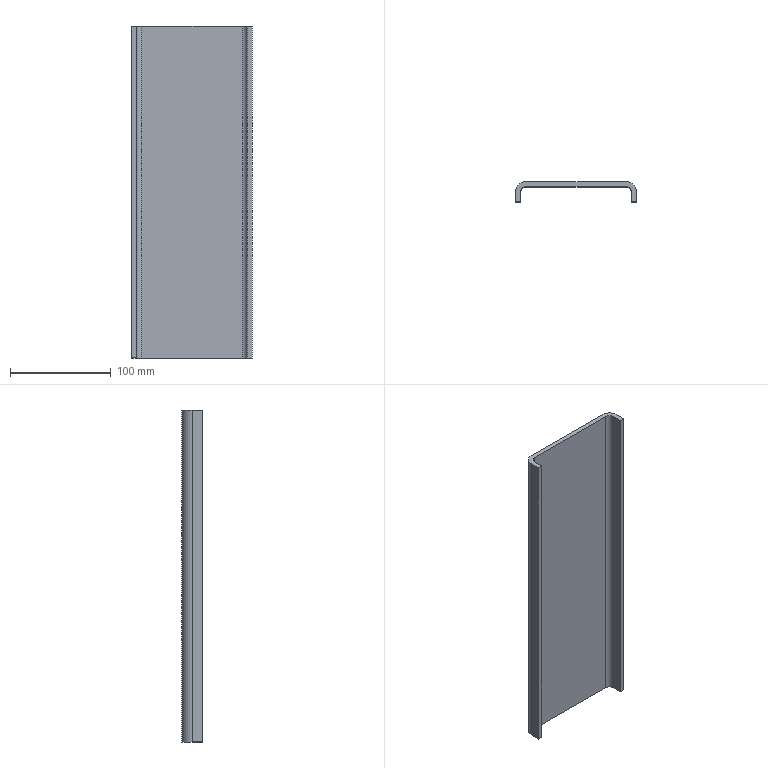Part | SolidWorks | features Extrusion 1, ICE 1 | 1 solid | 14 faces | box 120 x 20 x 330 mm | volume 236877 mm3 | plane 10 | cylinder 4 | commonest cylinder face diameters 10 x2 20 x2
STEP:
#1=CARTESIAN_POINT('',(115.,-20.,320.));
#2=VERTEX_POINT('',#1);
#3=CARTESIAN_POINT('',(115.,-20.,-10.));
#4=VERTEX_POINT('',#3);
#5=CARTESIAN_POINT('',(115.,-20.,320.));
#6=DIRECTION('',(0.,0.,-1.));
#7=VECTOR('',#6,1000.);
#8=LINE('',#5,#7);
#9=EDGE_CURVE('',#2,#4,#8,.T.);
#10=ORIENTED_EDGE('',*,*,#9,.T.);
#11=CARTESIAN_POINT('',(120.,-20.,-10.));
#12=VERTEX_POINT('',#11);
#13=CARTESIAN_POINT('',(120.,-20.,-10.));
#14=DIRECTION('',(-1.,0.,0.));
#15=VECTOR('',#14,1000.);
#16=LINE('',#13,#15);
#17=EDGE_CURVE('',#12,#4,#16,.T.);
#18=ORIENTED_EDGE('',*,*,#17,.F.);
#19=CARTESIAN_POINT('',(120.,-20.,320.));
#20=VERTEX_POINT('',#19);
#21=CARTESIAN_POINT('',(120.,-20.,320.));
#22=DIRECTION('',(0.,0.,-1.));
#23=VECTOR('',#22,1000.);
#24=LINE('',#21,#23);
#25=EDGE_CURVE('',#20,#12,#24,.T.);
#26=ORIENTED_EDGE('',*,*,#25,.F.);
#27=CARTESIAN_POINT('',(115.,-20.,320.));
#28=DIRECTION('',(1.,0.,0.));
#29=VECTOR('',#28,1000.);
#30=LINE('',#27,#29);
#31=EDGE_CURVE('',#2,#20,#30,.T.);
#32=ORIENTED_EDGE('',*,*,#31,.F.);
#33=EDGE_LOOP('',(#10,#18,#26,#32));
#34=FACE_OUTER_BOUND('',#33,.T.);
#35=CARTESIAN_POINT('',(115.,-20.,320.));
#36=DIRECTION('',(0.,1.,0.));
#37=DIRECTION('',(0.,0.,1.));
#38=AXIS2_PLACEMENT_3D('',#35,#36,#37);
#39=PLANE('',#38);
#40=ADVANCED_FACE('',(#34),#39,.F.);
#41=ORIENTED_EDGE('',*,*,#25,.T.);
#42=CARTESIAN_POINT('',(120.,-10.,-10.));
#43=VERTEX_POINT('',#42);
#44=CARTESIAN_POINT('',(120.,-10.,-10.));
#45=DIRECTION('',(0.,-1.,0.));
#46=VECTOR('',#45,1000.);
#47=LINE('',#44,#46);
#48=EDGE_CURVE('',#43,#12,#47,.T.);
#49=ORIENTED_EDGE('',*,*,#48,.F.);
#50=CARTESIAN_POINT('',(120.,-10.,320.));
#51=VERTEX_POINT('',#50);
#52=CARTESIAN_POINT('',(120.,-10.,320.));
#53=DIRECTION('',(0.,0.,-1.));
#54=VECTOR('',#53,1000.);
#55=LINE('',#52,#54);
#56=EDGE_CURVE('',#51,#43,#55,.T.);
#57=ORIENTED_EDGE('',*,*,#56,.F.);
#58=CARTESIAN_POINT('',(120.,-10.,320.));
#59=DIRECTION('',(0.,1.,0.));
#60=VECTOR('',#59,1000.);
#61=LINE('',#58,#60);
#62=EDGE_CURVE('',#20,#51,#61,.T.);
#63=ORIENTED_EDGE('',*,*,#62,.F.);
#64=EDGE_LOOP('',(#41,#49,#57,#63));
#65=FACE_OUTER_BOUND('',#64,.T.);
#66=CARTESIAN_POINT('',(120.,-10.,320.));
#67=DIRECTION('',(-1.,0.,0.));
#68=DIRECTION('',(0.,0.,1.));
#69=AXIS2_PLACEMENT_3D('',#66,#67,#68);
#70=PLANE('',#69);
#71=ADVANCED_FACE('',(#65),#70,.F.);
#72=ORIENTED_EDGE('',*,*,#56,.T.);
#73=CARTESIAN_POINT('',(110.,0.,-10.));
#74=VERTEX_POINT('',#73);
#75=CARTESIAN_POINT('',(110.,-10.,-10.));
#76=DIRECTION('',(0.,0.,-1.));
#77=DIRECTION('',(-1.,0.,0.));
#78=AXIS2_PLACEMENT_3D('',#75,#76,#77);
#79=CIRCLE('',#78,10.);
#80=EDGE_CURVE('',#74,#43,#79,.T.);
#81=ORIENTED_EDGE('',*,*,#80,.F.);
#82=CARTESIAN_POINT('',(110.,0.,320.));
#83=VERTEX_POINT('',#82);
#84=CARTESIAN_POINT('',(110.,0.,320.));
#85=DIRECTION('',(0.,0.,-1.));
#86=VECTOR('',#85,1000.);
#87=LINE('',#84,#86);
#88=EDGE_CURVE('',#83,#74,#87,.T.);
#89=ORIENTED_EDGE('',*,*,#88,.F.);
#90=CARTESIAN_POINT('',(110.,-10.,320.));
#91=DIRECTION('',(0.,0.,1.));
#92=DIRECTION('',(1.,0.,0.));
#93=AXIS2_PLACEMENT_3D('',#90,#91,#92);
#94=CIRCLE('',#93,10.);
#95=EDGE_CURVE('',#51,#83,#94,.T.);
#96=ORIENTED_EDGE('',*,*,#95,.F.);
#97=EDGE_LOOP('',(#72,#81,#89,#96));
#98=FACE_OUTER_BOUND('',#97,.T.);
#99=CARTESIAN_POINT('',(110.,-10.,320.));
#100=DIRECTION('',(0.,0.,-1.));
#101=DIRECTION('',(-1.,0.,0.));
#102=AXIS2_PLACEMENT_3D('',#99,#100,#101);
#103=CYLINDRICAL_SURFACE('',#102,10.);
#104=ADVANCED_FACE('',(#98),#103,.T.);
#105=ORIENTED_EDGE('',*,*,#88,.T.);
#106=CARTESIAN_POINT('',(10.,0.,-10.));
#107=VERTEX_POINT('',#106);
#108=CARTESIAN_POINT('',(10.,0.,-10.));
#109=DIRECTION('',(1.,0.,0.));
#110=VECTOR('',#109,1000.);
#111=LINE('',#108,#110);
#112=EDGE_CURVE('',#107,#74,#111,.T.);
#113=ORIENTED_EDGE('',*,*,#112,.F.);
#114=CARTESIAN_POINT('',(10.,0.,320.));
#115=VERTEX_POINT('',#114);
#116=CARTESIAN_POINT('',(10.,0.,320.));
#117=DIRECTION('',(0.,0.,-1.));
#118=VECTOR('',#117,1000.);
#119=LINE('',#116,#118);
#120=EDGE_CURVE('',#115,#107,#119,.T.);
#121=ORIENTED_EDGE('',*,*,#120,.F.);
#122=CARTESIAN_POINT('',(10.,0.,320.));
#123=DIRECTION('',(-1.,0.,0.));
#124=VECTOR('',#123,1000.);
#125=LINE('',#122,#124);
#126=EDGE_CURVE('',#83,#115,#125,.T.);
#127=ORIENTED_EDGE('',*,*,#126,.F.);
#128=EDGE_LOOP('',(#105,#113,#121,#127));
#129=FACE_OUTER_BOUND('',#128,.T.);
#130=CARTESIAN_POINT('',(10.,0.,320.));
#131=DIRECTION('',(0.,-1.,0.));
#132=DIRECTION('',(0.,0.,-1.));
#133=AXIS2_PLACEMENT_3D('',#130,#131,#132);
#134=PLANE('',#133);
#135=ADVANCED_FACE('',(#129),#134,.F.);
#136=ORIENTED_EDGE('',*,*,#120,.T.);
#137=CARTESIAN_POINT('',(0.,-10.,-10.));
#138=VERTEX_POINT('',#137);
#139=CARTESIAN_POINT('',(10.,-10.,-10.));
#140=DIRECTION('',(0.,0.,-1.));
#141=DIRECTION('',(-1.,0.,0.));
#142=AXIS2_PLACEMENT_3D('',#139,#140,#141);
#143=CIRCLE('',#142,10.);
#144=EDGE_CURVE('',#138,#107,#143,.T.);
#145=ORIENTED_EDGE('',*,*,#144,.F.);
#146=CARTESIAN_POINT('',(0.,-10.,320.));
#147=VERTEX_POINT('',#146);
#148=CARTESIAN_POINT('',(0.,-10.,320.));
#149=DIRECTION('',(0.,0.,-1.));
#150=VECTOR('',#149,1000.);
#151=LINE('',#148,#150);
#152=EDGE_CURVE('',#147,#138,#151,.T.);
#153=ORIENTED_EDGE('',*,*,#152,.F.);
#154=CARTESIAN_POINT('',(10.,-10.,320.));
#155=DIRECTION('',(0.,0.,1.));
#156=DIRECTION('',(1.,0.,0.));
#157=AXIS2_PLACEMENT_3D('',#154,#155,#156);
#158=CIRCLE('',#157,10.);
#159=EDGE_CURVE('',#115,#147,#158,.T.);
#160=ORIENTED_EDGE('',*,*,#159,.F.);
#161=EDGE_LOOP('',(#136,#145,#153,#160));
#162=FACE_OUTER_BOUND('',#161,.T.);
#163=CARTESIAN_POINT('',(10.,-10.,320.));
#164=DIRECTION('',(0.,0.,-1.));
#165=DIRECTION('',(-1.,0.,0.));
#166=AXIS2_PLACEMENT_3D('',#163,#164,#165);
#167=CYLINDRICAL_SURFACE('',#166,10.);
#168=ADVANCED_FACE('',(#162),#167,.T.);
#169=ORIENTED_EDGE('',*,*,#152,.T.);
#170=CARTESIAN_POINT('',(0.,-20.,-10.));
#171=VERTEX_POINT('',#170);
#172=CARTESIAN_POINT('',(0.,-20.,-10.));
#173=DIRECTION('',(0.,1.,0.));
#174=VECTOR('',#173,1000.);
#175=LINE('',#172,#174);
#176=EDGE_CURVE('',#171,#138,#175,.T.);
#177=ORIENTED_EDGE('',*,*,#176,.F.);
#178=CARTESIAN_POINT('',(0.,-20.,320.));
#179=VERTEX_POINT('',#178);
#180=CARTESIAN_POINT('',(0.,-20.,320.));
#181=DIRECTION('',(0.,0.,-1.));
#182=VECTOR('',#181,1000.);
#183=LINE('',#180,#182);
#184=EDGE_CURVE('',#179,#171,#183,.T.);
#185=ORIENTED_EDGE('',*,*,#184,.F.);
#186=CARTESIAN_POINT('',(0.,-10.,320.));
#187=DIRECTION('',(0.,-1.,0.));
#188=VECTOR('',#187,1000.);
#189=LINE('',#186,#188);
#190=EDGE_CURVE('',#147,#179,#189,.T.);
#191=ORIENTED_EDGE('',*,*,#190,.F.);
#192=EDGE_LOOP('',(#169,#177,#185,#191));
#193=FACE_OUTER_BOUND('',#192,.T.);
#194=CARTESIAN_POINT('',(0.,-10.,320.));
#195=DIRECTION('',(1.,0.,0.));
#196=DIRECTION('',(0.,1.,0.));
#197=AXIS2_PLACEMENT_3D('',#194,#195,#196);
#198=PLANE('',#197);
#199=ADVANCED_FACE('',(#193),#198,.F.);
#200=ORIENTED_EDGE('',*,*,#184,.T.);
#201=CARTESIAN_POINT('',(5.,-20.,-10.));
#202=VERTEX_POINT('',#201);
#203=CARTESIAN_POINT('',(5.,-20.,-10.));
#204=DIRECTION('',(-1.,0.,0.));
#205=VECTOR('',#204,1000.);
#206=LINE('',#203,#205);
#207=EDGE_CURVE('',#202,#171,#206,.T.);
#208=ORIENTED_EDGE('',*,*,#207,.F.);
#209=CARTESIAN_POINT('',(5.,-20.,320.));
#210=VERTEX_POINT('',#209);
#211=CARTESIAN_POINT('',(5.,-20.,320.));
#212=DIRECTION('',(0.,0.,-1.));
#213=VECTOR('',#212,1000.);
#214=LINE('',#211,#213);
#215=EDGE_CURVE('',#210,#202,#214,.T.);
#216=ORIENTED_EDGE('',*,*,#215,.F.);
#217=CARTESIAN_POINT('',(0.,-20.,320.));
#218=DIRECTION('',(1.,0.,0.));
#219=VECTOR('',#218,1000.);
#220=LINE('',#217,#219);
#221=EDGE_CURVE('',#179,#210,#220,.T.);
#222=ORIENTED_EDGE('',*,*,#221,.F.);
#223=EDGE_LOOP('',(#200,#208,#216,#222));
#224=FACE_OUTER_BOUND('',#223,.T.);
#225=CARTESIAN_POINT('',(0.,-20.,320.));
#226=DIRECTION('',(0.,1.,0.));
#227=DIRECTION('',(0.,0.,1.));
#228=AXIS2_PLACEMENT_3D('',#225,#226,#227);
#229=PLANE('',#228);
#230=ADVANCED_FACE('',(#224),#229,.F.);
#231=ORIENTED_EDGE('',*,*,#215,.T.);
#232=CARTESIAN_POINT('',(5.,-10.,-10.));
#233=VERTEX_POINT('',#232);
#234=CARTESIAN_POINT('',(5.,-10.,-10.));
#235=DIRECTION('',(0.,-1.,0.));
#236=VECTOR('',#235,1000.);
#237=LINE('',#234,#236);
#238=EDGE_CURVE('',#233,#202,#237,.T.);
#239=ORIENTED_EDGE('',*,*,#238,.F.);
#240=CARTESIAN_POINT('',(5.,-10.,320.));
#241=VERTEX_POINT('',#240);
#242=CARTESIAN_POINT('',(5.,-10.,320.));
#243=DIRECTION('',(0.,0.,-1.));
#244=VECTOR('',#243,1000.);
#245=LINE('',#242,#244);
#246=EDGE_CURVE('',#241,#233,#245,.T.);
#247=ORIENTED_EDGE('',*,*,#246,.F.);
#248=CARTESIAN_POINT('',(5.,-10.,320.));
#249=DIRECTION('',(0.,1.,0.));
#250=VECTOR('',#249,1000.);
#251=LINE('',#248,#250);
#252=EDGE_CURVE('',#210,#241,#251,.T.);
#253=ORIENTED_EDGE('',*,*,#252,.F.);
#254=EDGE_LOOP('',(#231,#239,#247,#253));
#255=FACE_OUTER_BOUND('',#254,.T.);
#256=CARTESIAN_POINT('',(5.,-10.,320.));
#257=DIRECTION('',(-1.,0.,0.));
#258=DIRECTION('',(0.,0.,1.));
#259=AXIS2_PLACEMENT_3D('',#256,#257,#258);
#260=PLANE('',#259);
#261=ADVANCED_FACE('',(#255),#260,.F.);
#262=ORIENTED_EDGE('',*,*,#246,.T.);
#263=CARTESIAN_POINT('',(10.,-5.,-10.));
#264=VERTEX_POINT('',#263);
#265=CARTESIAN_POINT('',(10.,-10.,-10.));
#266=DIRECTION('',(0.,0.,1.));
#267=DIRECTION('',(-1.,0.,0.));
#268=AXIS2_PLACEMENT_3D('',#265,#266,#267);
#269=CIRCLE('',#268,5.);
#270=EDGE_CURVE('',#264,#233,#269,.T.);
#271=ORIENTED_EDGE('',*,*,#270,.F.);
#272=CARTESIAN_POINT('',(10.,-5.,320.));
#273=VERTEX_POINT('',#272);
#274=CARTESIAN_POINT('',(10.,-5.,320.));
#275=DIRECTION('',(0.,0.,-1.));
#276=VECTOR('',#275,1000.);
#277=LINE('',#274,#276);
#278=EDGE_CURVE('',#273,#264,#277,.T.);
#279=ORIENTED_EDGE('',*,*,#278,.F.);
#280=CARTESIAN_POINT('',(10.,-10.,320.));
#281=DIRECTION('',(0.,0.,-1.));
#282=DIRECTION('',(1.,0.,0.));
#283=AXIS2_PLACEMENT_3D('',#280,#281,#282);
#284=CIRCLE('',#283,5.);
#285=EDGE_CURVE('',#241,#273,#284,.T.);
#286=ORIENTED_EDGE('',*,*,#285,.F.);
#287=EDGE_LOOP('',(#262,#271,#279,#286));
#288=FACE_OUTER_BOUND('',#287,.T.);
#289=CARTESIAN_POINT('',(10.,-10.,320.));
#290=DIRECTION('',(0.,0.,-1.));
#291=DIRECTION('',(-1.,0.,0.));
#292=AXIS2_PLACEMENT_3D('',#289,#290,#291);
#293=CYLINDRICAL_SURFACE('',#292,5.);
#294=ADVANCED_FACE('',(#288),#293,.F.);
#295=ORIENTED_EDGE('',*,*,#278,.T.);
#296=CARTESIAN_POINT('',(110.,-5.,-10.));
#297=VERTEX_POINT('',#296);
#298=CARTESIAN_POINT('',(110.,-5.,-10.));
#299=DIRECTION('',(-1.,0.,0.));
#300=VECTOR('',#299,1000.);
#301=LINE('',#298,#300);
#302=EDGE_CURVE('',#297,#264,#301,.T.);
#303=ORIENTED_EDGE('',*,*,#302,.F.);
#304=CARTESIAN_POINT('',(110.,-5.,320.));
#305=VERTEX_POINT('',#304);
#306=CARTESIAN_POINT('',(110.,-5.,320.));
#307=DIRECTION('',(0.,0.,-1.));
#308=VECTOR('',#307,1000.);
#309=LINE('',#306,#308);
#310=EDGE_CURVE('',#305,#297,#309,.T.);
#311=ORIENTED_EDGE('',*,*,#310,.F.);
#312=CARTESIAN_POINT('',(10.,-5.,320.));
#313=DIRECTION('',(1.,0.,0.));
#314=VECTOR('',#313,1000.);
#315=LINE('',#312,#314);
#316=EDGE_CURVE('',#273,#305,#315,.T.);
#317=ORIENTED_EDGE('',*,*,#316,.F.);
#318=EDGE_LOOP('',(#295,#303,#311,#317));
#319=FACE_OUTER_BOUND('',#318,.T.);
#320=CARTESIAN_POINT('',(10.,-5.,320.));
#321=DIRECTION('',(0.,1.,0.));
#322=DIRECTION('',(0.,0.,1.));
#323=AXIS2_PLACEMENT_3D('',#320,#321,#322);
#324=PLANE('',#323);
#325=ADVANCED_FACE('',(#319),#324,.F.);
#326=ORIENTED_EDGE('',*,*,#310,.T.);
#327=CARTESIAN_POINT('',(115.,-10.,-10.));
#328=VERTEX_POINT('',#327);
#329=CARTESIAN_POINT('',(110.,-10.,-10.));
#330=DIRECTION('',(0.,0.,1.));
#331=DIRECTION('',(-1.,0.,0.));
#332=AXIS2_PLACEMENT_3D('',#329,#330,#331);
#333=CIRCLE('',#332,5.);
#334=EDGE_CURVE('',#328,#297,#333,.T.);
#335=ORIENTED_EDGE('',*,*,#334,.F.);
#336=CARTESIAN_POINT('',(115.,-10.,320.));
#337=VERTEX_POINT('',#336);
#338=CARTESIAN_POINT('',(115.,-10.,320.));
#339=DIRECTION('',(0.,0.,-1.));
#340=VECTOR('',#339,1000.);
#341=LINE('',#338,#340);
#342=EDGE_CURVE('',#337,#328,#341,.T.);
#343=ORIENTED_EDGE('',*,*,#342,.F.);
#344=CARTESIAN_POINT('',(110.,-10.,320.));
#345=DIRECTION('',(0.,0.,-1.));
#346=DIRECTION('',(1.,0.,0.));
#347=AXIS2_PLACEMENT_3D('',#344,#345,#346);
#348=CIRCLE('',#347,5.);
#349=EDGE_CURVE('',#305,#337,#348,.T.);
#350=ORIENTED_EDGE('',*,*,#349,.F.);
#351=EDGE_LOOP('',(#326,#335,#343,#350));
#352=FACE_OUTER_BOUND('',#351,.T.);
#353=CARTESIAN_POINT('',(110.,-10.,320.));
#354=DIRECTION('',(0.,0.,-1.));
#355=DIRECTION('',(-1.,0.,0.));
#356=AXIS2_PLACEMENT_3D('',#353,#354,#355);
#357=CYLINDRICAL_SURFACE('',#356,5.);
#358=ADVANCED_FACE('',(#352),#357,.F.);
#359=ORIENTED_EDGE('',*,*,#342,.T.);
#360=CARTESIAN_POINT('',(115.,-20.,-10.));
#361=DIRECTION('',(0.,1.,0.));
#362=VECTOR('',#361,1000.);
#363=LINE('',#360,#362);
#364=EDGE_CURVE('',#4,#328,#363,.T.);
#365=ORIENTED_EDGE('',*,*,#364,.F.);
#366=ORIENTED_EDGE('',*,*,#9,.F.);
#367=CARTESIAN_POINT('',(115.,-10.,320.));
#368=DIRECTION('',(0.,-1.,0.));
#369=VECTOR('',#368,1000.);
#370=LINE('',#367,#369);
#371=EDGE_CURVE('',#337,#2,#370,.T.);
#372=ORIENTED_EDGE('',*,*,#371,.F.);
#373=EDGE_LOOP('',(#359,#365,#366,#372));
#374=FACE_OUTER_BOUND('',#373,.T.);
#375=CARTESIAN_POINT('',(115.,-10.,320.));
#376=DIRECTION('',(1.,0.,0.));
#377=DIRECTION('',(0.,1.,0.));
#378=AXIS2_PLACEMENT_3D('',#375,#376,#377);
#379=PLANE('',#378);
#380=ADVANCED_FACE('',(#374),#379,.F.);
#381=ORIENTED_EDGE('',*,*,#31,.T.);
#382=ORIENTED_EDGE('',*,*,#62,.T.);
#383=ORIENTED_EDGE('',*,*,#95,.T.);
#384=ORIENTED_EDGE('',*,*,#126,.T.);
#385=ORIENTED_EDGE('',*,*,#159,.T.);
#386=ORIENTED_EDGE('',*,*,#190,.T.);
#387=ORIENTED_EDGE('',*,*,#221,.T.);
#388=ORIENTED_EDGE('',*,*,#252,.T.);
#389=ORIENTED_EDGE('',*,*,#285,.T.);
#390=ORIENTED_EDGE('',*,*,#316,.T.);
#391=ORIENTED_EDGE('',*,*,#349,.T.);
#392=ORIENTED_EDGE('',*,*,#371,.T.);
#393=EDGE_LOOP('',(#381,#382,#383,#384,#385,#386,#387,#388,#389,#390,#391,#392));
#394=FACE_OUTER_BOUND('',#393,.T.);
#395=CARTESIAN_POINT('',(110.,-10.,320.));
#396=DIRECTION('',(0.,0.,1.));
#397=DIRECTION('',(1.,0.,0.));
#398=AXIS2_PLACEMENT_3D('',#395,#396,#397);
#399=PLANE('',#398);
#400=ADVANCED_FACE('',(#394),#399,.T.);
#401=ORIENTED_EDGE('',*,*,#48,.T.);
#402=ORIENTED_EDGE('',*,*,#17,.T.);
#403=ORIENTED_EDGE('',*,*,#364,.T.);
#404=ORIENTED_EDGE('',*,*,#334,.T.);
#405=ORIENTED_EDGE('',*,*,#302,.T.);
#406=ORIENTED_EDGE('',*,*,#270,.T.);
#407=ORIENTED_EDGE('',*,*,#238,.T.);
#408=ORIENTED_EDGE('',*,*,#207,.T.);
#409=ORIENTED_EDGE('',*,*,#176,.T.);
#410=ORIENTED_EDGE('',*,*,#144,.T.);
#411=ORIENTED_EDGE('',*,*,#112,.T.);
#412=ORIENTED_EDGE('',*,*,#80,.T.);
#413=EDGE_LOOP('',(#401,#402,#403,#404,#405,#406,#407,#408,#409,#410,#411,#412));
#414=FACE_OUTER_BOUND('',#413,.T.);
#415=CARTESIAN_POINT('',(110.,-10.,-10.));
#416=DIRECTION('',(0.,0.,-1.));
#417=DIRECTION('',(-1.,0.,0.));
#418=AXIS2_PLACEMENT_3D('',#415,#416,#417);
#419=PLANE('',#418);
#420=ADVANCED_FACE('',(#414),#419,.T.);
#421=CLOSED_SHELL('',(#40,#71,#104,#135,#168,#199,#230,#261,#294,#325,#358,#380,#400,#420));
#422=MANIFOLD_SOLID_BREP('',#421);
#423=CARTESIAN_POINT('',(0.,0.,0.));
#424=DIRECTION('',(0.,0.,1.));
#425=DIRECTION('',(1.,0.,0.));
#426=AXIS2_PLACEMENT_3D('',#423,#424,#425);
#427=(LENGTH_UNIT()NAMED_UNIT(*)SI_UNIT(.MILLI.,.METRE.));
#428=UNCERTAINTY_MEASURE_WITH_UNIT(LENGTH_MEASURE(0.00001),#427,'','');
#429=(NAMED_UNIT(*)PLANE_ANGLE_UNIT()SI_UNIT($,.RADIAN.));
#430=(NAMED_UNIT(*)SI_UNIT($,.STERADIAN.)SOLID_ANGLE_UNIT());
#431=(GEOMETRIC_REPRESENTATION_CONTEXT(3)GLOBAL_UNCERTAINTY_ASSIGNED_CONTEXT((#428))GLOBAL_UNIT_ASSIGNED_CONTEXT((#427,#429,#430))REPRESENTATION_CONTEXT('',''));
#432=ADVANCED_BREP_SHAPE_REPRESENTATION('',(#422,#426),#431);